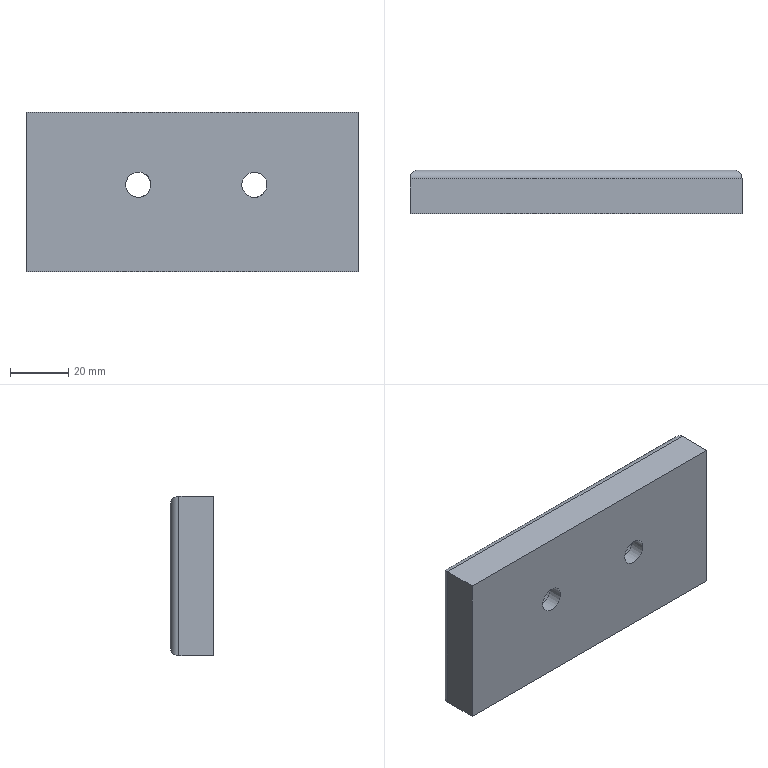Part | STEP file | 1_id1606_x_t | 1 solid | 16 faces | box 114.3 x 15 x 55 mm | volume 89525 mm3 | plane 8 | cylinder 8 | commonest cylinder face diameters 6 x4 8.7 x2 15 x2
STEP:
#1=CARTESIAN_POINT('',(0.,0.,0.));
#2=DIRECTION('',(0.,0.,1.));
#3=DIRECTION('',(1.,0.,0.));
#4=AXIS2_PLACEMENT_3D('',#1,#2,#3);
#5=CARTESIAN_POINT('',(661.35,282.376,-11.278));
#6=VERTEX_POINT('',#5);
#7=CARTESIAN_POINT('',(553.05,282.376,-11.278));
#8=VERTEX_POINT('',#7);
#9=CARTESIAN_POINT('',(661.35,282.376,-11.278));
#10=DIRECTION('',(-1.,0.,0.));
#11=VECTOR('',#10,1.);
#12=LINE('',#9,#11);
#13=CARTESIAN_POINT('',(606.2,282.376,-8.278));
#14=DIRECTION('',(0.,1.,0.));
#15=DIRECTION('',(0.,0.,-1.));
#16=AXIS2_PLACEMENT_3D('',#13,#14,#15);
#17=PLANE('',#16);
#18=CARTESIAN_POINT('',(3.,-55.15));
#19=DIRECTION('',(0.,1.));
#20=VECTOR('',#19,1.);
#21=LINE('',#18,#20);
#22=(GEOMETRIC_REPRESENTATION_CONTEXT(2)PARAMETRIC_REPRESENTATION_CONTEXT()REPRESENTATION_CONTEXT('',''));
#23=DEFINITIONAL_REPRESENTATION('',(#21),#22);
#24=PCURVE('',#17,#23);
#25=CARTESIAN_POINT('',(606.2,279.376,-11.278));
#26=DIRECTION('',(1.,0.,0.));
#27=DIRECTION('',(0.,0.,-1.));
#28=AXIS2_PLACEMENT_3D('',#25,#26,#27);
#29=CYLINDRICAL_SURFACE('',#28,3.);
#30=CARTESIAN_POINT('',(1.571,55.15));
#31=DIRECTION('',(0.,-1.));
#32=VECTOR('',#31,1.);
#33=LINE('',#30,#32);
#34=(GEOMETRIC_REPRESENTATION_CONTEXT(2)PARAMETRIC_REPRESENTATION_CONTEXT()REPRESENTATION_CONTEXT('',''));
#35=DEFINITIONAL_REPRESENTATION('',(#33),#34);
#36=PCURVE('',#29,#35);
#37=SURFACE_CURVE('',#12,(#24,#36),.PCURVE_S1.);
#38=EDGE_CURVE('',#6,#8,#37,.T.);
#39=ORIENTED_EDGE('',*,*,#38,.F.);
#40=CARTESIAN_POINT('',(661.35,282.376,-60.278));
#41=VERTEX_POINT('',#40);
#42=CARTESIAN_POINT('',(661.35,282.376,-60.278));
#43=DIRECTION('',(0.,0.,1.));
#44=VECTOR('',#43,1.);
#45=LINE('',#42,#44);
#46=CARTESIAN_POINT('',(52.,-55.15));
#47=DIRECTION('',(-1.,0.));
#48=VECTOR('',#47,1.);
#49=LINE('',#46,#48);
#50=(GEOMETRIC_REPRESENTATION_CONTEXT(2)PARAMETRIC_REPRESENTATION_CONTEXT()REPRESENTATION_CONTEXT('',''));
#51=DEFINITIONAL_REPRESENTATION('',(#49),#50);
#52=PCURVE('',#17,#51);
#53=CARTESIAN_POINT('',(661.35,279.376,-8.278));
#54=DIRECTION('',(0.,0.,-1.));
#55=DIRECTION('',(-1.,0.,0.));
#56=AXIS2_PLACEMENT_3D('',#53,#54,#55);
#57=CYLINDRICAL_SURFACE('',#56,3.);
#58=CARTESIAN_POINT('',(1.571,52.));
#59=DIRECTION('',(0.,-1.));
#60=VECTOR('',#59,1.);
#61=LINE('',#58,#60);
#62=(GEOMETRIC_REPRESENTATION_CONTEXT(2)PARAMETRIC_REPRESENTATION_CONTEXT()REPRESENTATION_CONTEXT('',''));
#63=DEFINITIONAL_REPRESENTATION('',(#61),#62);
#64=PCURVE('',#57,#63);
#65=SURFACE_CURVE('',#45,(#52,#64),.PCURVE_S1.);
#66=EDGE_CURVE('',#41,#6,#65,.T.);
#67=ORIENTED_EDGE('',*,*,#66,.F.);
#68=CARTESIAN_POINT('',(553.05,282.376,-60.278));
#69=VERTEX_POINT('',#68);
#70=CARTESIAN_POINT('',(553.05,282.376,-60.278));
#71=DIRECTION('',(1.,0.,0.));
#72=VECTOR('',#71,1.);
#73=LINE('',#70,#72);
#74=CARTESIAN_POINT('',(52.,53.15));
#75=DIRECTION('',(0.,-1.));
#76=VECTOR('',#75,1.);
#77=LINE('',#74,#76);
#78=(GEOMETRIC_REPRESENTATION_CONTEXT(2)PARAMETRIC_REPRESENTATION_CONTEXT()REPRESENTATION_CONTEXT('',''));
#79=DEFINITIONAL_REPRESENTATION('',(#77),#78);
#80=PCURVE('',#17,#79);
#81=CARTESIAN_POINT('',(606.2,279.376,-60.278));
#82=DIRECTION('',(-1.,0.,0.));
#83=DIRECTION('',(0.,0.,1.));
#84=AXIS2_PLACEMENT_3D('',#81,#82,#83);
#85=CYLINDRICAL_SURFACE('',#84,3.);
#86=CARTESIAN_POINT('',(1.571,53.15));
#87=DIRECTION('',(0.,-1.));
#88=VECTOR('',#87,1.);
#89=LINE('',#86,#88);
#90=(GEOMETRIC_REPRESENTATION_CONTEXT(2)PARAMETRIC_REPRESENTATION_CONTEXT()REPRESENTATION_CONTEXT('',''));
#91=DEFINITIONAL_REPRESENTATION('',(#89),#90);
#92=PCURVE('',#85,#91);
#93=SURFACE_CURVE('',#73,(#80,#92),.PCURVE_S1.);
#94=EDGE_CURVE('',#69,#41,#93,.T.);
#95=ORIENTED_EDGE('',*,*,#94,.F.);
#96=CARTESIAN_POINT('',(553.05,282.376,-11.278));
#97=DIRECTION('',(0.,0.,-1.));
#98=VECTOR('',#97,1.);
#99=LINE('',#96,#98);
#100=CARTESIAN_POINT('',(3.,53.15));
#101=DIRECTION('',(1.,0.));
#102=VECTOR('',#101,1.);
#103=LINE('',#100,#102);
#104=(GEOMETRIC_REPRESENTATION_CONTEXT(2)PARAMETRIC_REPRESENTATION_CONTEXT()REPRESENTATION_CONTEXT('',''));
#105=DEFINITIONAL_REPRESENTATION('',(#103),#104);
#106=PCURVE('',#17,#105);
#107=CARTESIAN_POINT('',(553.05,279.376,-8.278));
#108=DIRECTION('',(0.,0.,-1.));
#109=DIRECTION('',(-1.,0.,0.));
#110=AXIS2_PLACEMENT_3D('',#107,#108,#109);
#111=CYLINDRICAL_SURFACE('',#110,3.);
#112=CARTESIAN_POINT('',(1.571,3.));
#113=DIRECTION('',(0.,1.));
#114=VECTOR('',#113,1.);
#115=LINE('',#112,#114);
#116=(GEOMETRIC_REPRESENTATION_CONTEXT(2)PARAMETRIC_REPRESENTATION_CONTEXT()REPRESENTATION_CONTEXT('',''));
#117=DEFINITIONAL_REPRESENTATION('',(#115),#116);
#118=PCURVE('',#111,#117);
#119=SURFACE_CURVE('',#99,(#106,#118),.PCURVE_S1.);
#120=EDGE_CURVE('',#8,#69,#119,.T.);
#121=ORIENTED_EDGE('',*,*,#120,.F.);
#122=EDGE_LOOP('',(#39,#67,#95,#121));
#123=FACE_BOUND('',#122,.T.);
#124=CARTESIAN_POINT('',(628.7,282.376,-25.778));
#125=VERTEX_POINT('',#124);
#126=CARTESIAN_POINT('',(628.7,282.376,-33.278));
#127=DIRECTION('',(0.,-1.,0.));
#128=DIRECTION('',(0.,0.,1.));
#129=AXIS2_PLACEMENT_3D('',#126,#127,#128);
#130=CIRCLE('',#129,7.5);
#131=CARTESIAN_POINT('',(17.5,-22.5));
#132=CARTESIAN_POINT('',(17.5,-9.51));
#133=CARTESIAN_POINT('',(28.75,-16.005));
#134=CARTESIAN_POINT('',(40.,-22.5));
#135=CARTESIAN_POINT('',(28.75,-28.995));
#136=CARTESIAN_POINT('',(17.5,-35.49));
#137=CARTESIAN_POINT('',(17.5,-22.5));
#138=(BOUNDED_CURVE()B_SPLINE_CURVE(2,(#131,#132,#133,#134,#135,#136,#137),.UNSPECIFIED.,.T.,.F.)B_SPLINE_CURVE_WITH_KNOTS((1,2,2,2,2,1),(-2.094,0.,2.094,4.189,6.283,8.378),.UNSPECIFIED.)CURVE()GEOMETRIC_REPRESENTATION_ITEM()RATIONAL_B_SPLINE_CURVE((1.,0.5,1.,0.5,1.,0.5,1.))REPRESENTATION_ITEM(''));
#139=(GEOMETRIC_REPRESENTATION_CONTEXT(2)PARAMETRIC_REPRESENTATION_CONTEXT()REPRESENTATION_CONTEXT('',''));
#140=DEFINITIONAL_REPRESENTATION('',(#138),#139);
#141=PCURVE('',#17,#140);
#142=CARTESIAN_POINT('',(628.7,272.376,-33.278));
#143=DIRECTION('',(0.,-1.,0.));
#144=DIRECTION('',(1.,0.,0.));
#145=AXIS2_PLACEMENT_3D('',#142,#143,#144);
#146=CYLINDRICAL_SURFACE('',#145,7.5);
#147=CARTESIAN_POINT('',(1.571,-10.));
#148=DIRECTION('',(1.,0.));
#149=VECTOR('',#148,1.);
#150=LINE('',#147,#149);
#151=(GEOMETRIC_REPRESENTATION_CONTEXT(2)PARAMETRIC_REPRESENTATION_CONTEXT()REPRESENTATION_CONTEXT('',''));
#152=DEFINITIONAL_REPRESENTATION('',(#150),#151);
#153=PCURVE('',#146,#152);
#154=SURFACE_CURVE('',#130,(#141,#153),.PCURVE_S1.);
#155=EDGE_CURVE('',#125,#125,#154,.T.);
#156=ORIENTED_EDGE('',*,*,#155,.T.);
#157=EDGE_LOOP('',(#156));
#158=FACE_BOUND('',#157,.T.);
#159=CARTESIAN_POINT('',(581.2,282.376,-33.278));
#160=VERTEX_POINT('',#159);
#161=CARTESIAN_POINT('',(588.7,282.376,-33.278));
#162=DIRECTION('',(0.,-1.,0.));
#163=DIRECTION('',(-1.,0.,0.));
#164=AXIS2_PLACEMENT_3D('',#161,#162,#163);
#165=CIRCLE('',#164,7.5);
#166=CARTESIAN_POINT('',(25.,25.));
#167=CARTESIAN_POINT('',(37.99,25.));
#168=CARTESIAN_POINT('',(31.495,13.75));
#169=CARTESIAN_POINT('',(25.,2.5));
#170=CARTESIAN_POINT('',(18.505,13.75));
#171=CARTESIAN_POINT('',(12.01,25.));
#172=CARTESIAN_POINT('',(25.,25.));
#173=(BOUNDED_CURVE()B_SPLINE_CURVE(2,(#166,#167,#168,#169,#170,#171,#172),.UNSPECIFIED.,.T.,.F.)B_SPLINE_CURVE_WITH_KNOTS((1,2,2,2,2,1),(-2.094,0.,2.094,4.189,6.283,8.378),.UNSPECIFIED.)CURVE()GEOMETRIC_REPRESENTATION_ITEM()RATIONAL_B_SPLINE_CURVE((1.,0.5,1.,0.5,1.,0.5,1.))REPRESENTATION_ITEM(''));
#174=(GEOMETRIC_REPRESENTATION_CONTEXT(2)PARAMETRIC_REPRESENTATION_CONTEXT()REPRESENTATION_CONTEXT('',''));
#175=DEFINITIONAL_REPRESENTATION('',(#173),#174);
#176=PCURVE('',#17,#175);
#177=CARTESIAN_POINT('',(588.7,272.376,-33.278));
#178=DIRECTION('',(0.,-1.,0.));
#179=DIRECTION('',(1.,0.,0.));
#180=AXIS2_PLACEMENT_3D('',#177,#178,#179);
#181=CYLINDRICAL_SURFACE('',#180,7.5);
#182=CARTESIAN_POINT('',(3.142,-10.));
#183=DIRECTION('',(1.,0.));
#184=VECTOR('',#183,1.);
#185=LINE('',#182,#184);
#186=(GEOMETRIC_REPRESENTATION_CONTEXT(2)PARAMETRIC_REPRESENTATION_CONTEXT()REPRESENTATION_CONTEXT('',''));
#187=DEFINITIONAL_REPRESENTATION('',(#185),#186);
#188=PCURVE('',#181,#187);
#189=SURFACE_CURVE('',#165,(#176,#188),.PCURVE_S1.);
#190=EDGE_CURVE('',#160,#160,#189,.T.);
#191=ORIENTED_EDGE('',*,*,#190,.T.);
#192=EDGE_LOOP('',(#191));
#193=FACE_BOUND('',#192,.T.);
#194=ADVANCED_FACE('',(#123,#158,#193),#17,.T.);
#195=CARTESIAN_POINT('',(550.05,279.376,-63.278));
#196=VERTEX_POINT('',#195);
#197=CARTESIAN_POINT('',(550.05,279.376,-8.278));
#198=VERTEX_POINT('',#197);
#199=CARTESIAN_POINT('',(550.05,279.376,-63.278));
#200=DIRECTION('',(0.,0.,1.));
#201=VECTOR('',#200,1.);
#202=LINE('',#199,#201);
#203=CARTESIAN_POINT('',(0.,55.));
#204=DIRECTION('',(0.,-1.));
#205=VECTOR('',#204,1.);
#206=LINE('',#203,#205);
#207=(GEOMETRIC_REPRESENTATION_CONTEXT(2)PARAMETRIC_REPRESENTATION_CONTEXT()REPRESENTATION_CONTEXT('',''));
#208=DEFINITIONAL_REPRESENTATION('',(#206),#207);
#209=PCURVE('',#111,#208);
#210=CARTESIAN_POINT('',(550.05,274.876,-8.278));
#211=DIRECTION('',(-1.,0.,0.));
#212=DIRECTION('',(0.,0.,1.));
#213=AXIS2_PLACEMENT_3D('',#210,#211,#212);
#214=PLANE('',#213);
#215=CARTESIAN_POINT('',(-55.,4.5));
#216=DIRECTION('',(1.,0.));
#217=VECTOR('',#216,1.);
#218=LINE('',#215,#217);
#219=(GEOMETRIC_REPRESENTATION_CONTEXT(2)PARAMETRIC_REPRESENTATION_CONTEXT()REPRESENTATION_CONTEXT('',''));
#220=DEFINITIONAL_REPRESENTATION('',(#218),#219);
#221=PCURVE('',#214,#220);
#222=SURFACE_CURVE('',#202,(#209,#221),.PCURVE_S1.);
#223=EDGE_CURVE('',#196,#198,#222,.T.);
#224=ORIENTED_EDGE('',*,*,#223,.T.);
#225=CARTESIAN_POINT('',(553.05,279.376,-11.278));
#226=DIRECTION('',(-0.7071,0.,-0.7071));
#227=DIRECTION('',(0.7071,0.,-0.7071));
#228=AXIS2_PLACEMENT_3D('',#225,#226,#227);
#229=ELLIPSE('',#228,4.243,3.);
#230=CARTESIAN_POINT('',(0.,0.));
#231=CARTESIAN_POINT('',(0.0238,-0.00000647));
#232=CARTESIAN_POINT('',(0.0714,0.005103));
#233=CARTESIAN_POINT('',(0.1428,0.02801));
#234=CARTESIAN_POINT('',(0.2142,0.06607));
#235=CARTESIAN_POINT('',(0.2856,0.1191));
#236=CARTESIAN_POINT('',(0.357,0.1868));
#237=CARTESIAN_POINT('',(0.4284,0.2688));
#238=CARTESIAN_POINT('',(0.4998,0.3647));
#239=CARTESIAN_POINT('',(0.5712,0.4741));
#240=CARTESIAN_POINT('',(0.6426,0.5963));
#241=CARTESIAN_POINT('',(0.714,0.7308));
#242=CARTESIAN_POINT('',(0.7854,0.8769));
#243=CARTESIAN_POINT('',(0.8568,1.034));
#244=CARTESIAN_POINT('',(0.9282,1.201));
#245=CARTESIAN_POINT('',(0.9996,1.377));
#246=CARTESIAN_POINT('',(1.071,1.561));
#247=CARTESIAN_POINT('',(1.142,1.753));
#248=CARTESIAN_POINT('',(1.214,1.951));
#249=CARTESIAN_POINT('',(1.285,2.154));
#250=CARTESIAN_POINT('',(1.357,2.362));
#251=CARTESIAN_POINT('',(1.428,2.573));
#252=CARTESIAN_POINT('',(1.499,2.786));
#253=CARTESIAN_POINT('',(1.547,2.929));
#254=CARTESIAN_POINT('',(1.571,3.));
#255=B_SPLINE_CURVE_WITH_KNOTS('',3,(#230,#231,#232,#233,#234,#235,#236,#237,#238,#239,#240,#241,#242,#243,#244,#245,#246,#247,#248,#249,#250,#251,#252,#253,#254),.UNSPECIFIED.,.F.,.F.,(4,1,1,1,1,1,1,1,1,1,1,1,1,1,1,1,1,1,1,1,1,1,4),(3.142,3.213,3.284,3.356,3.427,3.499,3.57,3.641,3.713,3.784,3.856,3.927,3.998,4.07,4.141,4.213,4.284,4.355,4.427,4.498,4.57,4.641,4.712),.QUASI_UNIFORM_KNOTS.);
#256=(GEOMETRIC_REPRESENTATION_CONTEXT(2)PARAMETRIC_REPRESENTATION_CONTEXT()REPRESENTATION_CONTEXT('',''));
#257=DEFINITIONAL_REPRESENTATION('',(#255),#256);
#258=PCURVE('',#111,#257);
#259=CARTESIAN_POINT('',(3.142,-56.15));
#260=CARTESIAN_POINT('',(3.118,-56.15));
#261=CARTESIAN_POINT('',(3.07,-56.145));
#262=CARTESIAN_POINT('',(2.999,-56.122));
#263=CARTESIAN_POINT('',(2.927,-56.084));
#264=CARTESIAN_POINT('',(2.856,-56.031));
#265=CARTESIAN_POINT('',(2.785,-55.963));
#266=CARTESIAN_POINT('',(2.713,-55.881));
#267=CARTESIAN_POINT('',(2.642,-55.785));
#268=CARTESIAN_POINT('',(2.57,-55.676));
#269=CARTESIAN_POINT('',(2.499,-55.554));
#270=CARTESIAN_POINT('',(2.428,-55.419));
#271=CARTESIAN_POINT('',(2.356,-55.273));
#272=CARTESIAN_POINT('',(2.285,-55.116));
#273=CARTESIAN_POINT('',(2.213,-54.949));
#274=CARTESIAN_POINT('',(2.142,-54.773));
#275=CARTESIAN_POINT('',(2.071,-54.589));
#276=CARTESIAN_POINT('',(1.999,-54.397));
#277=CARTESIAN_POINT('',(1.928,-54.199));
#278=CARTESIAN_POINT('',(1.856,-53.996));
#279=CARTESIAN_POINT('',(1.785,-53.788));
#280=CARTESIAN_POINT('',(1.714,-53.577));
#281=CARTESIAN_POINT('',(1.642,-53.364));
#282=CARTESIAN_POINT('',(1.595,-53.221));
#283=CARTESIAN_POINT('',(1.571,-53.15));
#284=B_SPLINE_CURVE_WITH_KNOTS('',3,(#259,#260,#261,#262,#263,#264,#265,#266,#267,#268,#269,#270,#271,#272,#273,#274,#275,#276,#277,#278,#279,#280,#281,#282,#283),.UNSPECIFIED.,.F.,.F.,(4,1,1,1,1,1,1,1,1,1,1,1,1,1,1,1,1,1,1,1,1,1,4),(3.142,3.213,3.284,3.356,3.427,3.499,3.57,3.641,3.713,3.784,3.856,3.927,3.998,4.07,4.141,4.213,4.284,4.355,4.427,4.498,4.57,4.641,4.712),.QUASI_UNIFORM_KNOTS.);
#285=(GEOMETRIC_REPRESENTATION_CONTEXT(2)PARAMETRIC_REPRESENTATION_CONTEXT()REPRESENTATION_CONTEXT('',''));
#286=DEFINITIONAL_REPRESENTATION('',(#284),#285);
#287=PCURVE('',#29,#286);
#288=SURFACE_CURVE('',#229,(#258,#287),.PCURVE_S1.);
#289=EDGE_CURVE('',#198,#8,#288,.T.);
#290=ORIENTED_EDGE('',*,*,#289,.T.);
#291=ORIENTED_EDGE('',*,*,#120,.T.);
#292=CARTESIAN_POINT('',(553.05,279.376,-60.278));
#293=DIRECTION('',(0.7071,0.,-0.7071));
#294=DIRECTION('',(-0.7071,0.,-0.7071));
#295=AXIS2_PLACEMENT_3D('',#292,#293,#294);
#296=ELLIPSE('',#295,4.243,3.);
#297=CARTESIAN_POINT('',(0.,55.));
#298=CARTESIAN_POINT('',(0.0238,55.));
#299=CARTESIAN_POINT('',(0.0714,54.995));
#300=CARTESIAN_POINT('',(0.1428,54.972));
#301=CARTESIAN_POINT('',(0.2142,54.934));
#302=CARTESIAN_POINT('',(0.2856,54.881));
#303=CARTESIAN_POINT('',(0.357,54.813));
#304=CARTESIAN_POINT('',(0.4284,54.731));
#305=CARTESIAN_POINT('',(0.4998,54.635));
#306=CARTESIAN_POINT('',(0.5712,54.526));
#307=CARTESIAN_POINT('',(0.6426,54.404));
#308=CARTESIAN_POINT('',(0.714,54.269));
#309=CARTESIAN_POINT('',(0.7854,54.123));
#310=CARTESIAN_POINT('',(0.8568,53.966));
#311=CARTESIAN_POINT('',(0.9282,53.799));
#312=CARTESIAN_POINT('',(0.9996,53.623));
#313=CARTESIAN_POINT('',(1.071,53.439));
#314=CARTESIAN_POINT('',(1.142,53.247));
#315=CARTESIAN_POINT('',(1.214,53.049));
#316=CARTESIAN_POINT('',(1.285,52.846));
#317=CARTESIAN_POINT('',(1.357,52.638));
#318=CARTESIAN_POINT('',(1.428,52.427));
#319=CARTESIAN_POINT('',(1.499,52.214));
#320=CARTESIAN_POINT('',(1.547,52.071));
#321=CARTESIAN_POINT('',(1.571,52.));
#322=B_SPLINE_CURVE_WITH_KNOTS('',3,(#297,#298,#299,#300,#301,#302,#303,#304,#305,#306,#307,#308,#309,#310,#311,#312,#313,#314,#315,#316,#317,#318,#319,#320,#321),.UNSPECIFIED.,.F.,.F.,(4,1,1,1,1,1,1,1,1,1,1,1,1,1,1,1,1,1,1,1,1,1,4),(0.,0.0714,0.1428,0.2142,0.2856,0.357,0.4284,0.4998,0.5712,0.6426,0.714,0.7854,0.8568,0.9282,0.9996,1.071,1.142,1.214,1.285,1.357,1.428,1.499,1.571),.QUASI_UNIFORM_KNOTS.);
#323=(GEOMETRIC_REPRESENTATION_CONTEXT(2)PARAMETRIC_REPRESENTATION_CONTEXT()REPRESENTATION_CONTEXT('',''));
#324=DEFINITIONAL_REPRESENTATION('',(#322),#323);
#325=PCURVE('',#111,#324);
#326=CARTESIAN_POINT('',(3.142,56.15));
#327=CARTESIAN_POINT('',(3.118,56.15));
#328=CARTESIAN_POINT('',(3.07,56.145));
#329=CARTESIAN_POINT('',(2.999,56.122));
#330=CARTESIAN_POINT('',(2.927,56.084));
#331=CARTESIAN_POINT('',(2.856,56.031));
#332=CARTESIAN_POINT('',(2.785,55.963));
#333=CARTESIAN_POINT('',(2.713,55.881));
#334=CARTESIAN_POINT('',(2.642,55.785));
#335=CARTESIAN_POINT('',(2.57,55.676));
#336=CARTESIAN_POINT('',(2.499,55.554));
#337=CARTESIAN_POINT('',(2.428,55.419));
#338=CARTESIAN_POINT('',(2.356,55.273));
#339=CARTESIAN_POINT('',(2.285,55.116));
#340=CARTESIAN_POINT('',(2.213,54.949));
#341=CARTESIAN_POINT('',(2.142,54.773));
#342=CARTESIAN_POINT('',(2.071,54.589));
#343=CARTESIAN_POINT('',(1.999,54.397));
#344=CARTESIAN_POINT('',(1.928,54.199));
#345=CARTESIAN_POINT('',(1.856,53.996));
#346=CARTESIAN_POINT('',(1.785,53.788));
#347=CARTESIAN_POINT('',(1.714,53.577));
#348=CARTESIAN_POINT('',(1.642,53.364));
#349=CARTESIAN_POINT('',(1.595,53.221));
#350=CARTESIAN_POINT('',(1.571,53.15));
#351=B_SPLINE_CURVE_WITH_KNOTS('',3,(#326,#327,#328,#329,#330,#331,#332,#333,#334,#335,#336,#337,#338,#339,#340,#341,#342,#343,#344,#345,#346,#347,#348,#349,#350),.UNSPECIFIED.,.F.,.F.,(4,1,1,1,1,1,1,1,1,1,1,1,1,1,1,1,1,1,1,1,1,1,4),(0.,0.0714,0.1428,0.2142,0.2856,0.357,0.4284,0.4998,0.5712,0.6426,0.714,0.7854,0.8568,0.9282,0.9996,1.071,1.142,1.214,1.285,1.357,1.428,1.499,1.571),.QUASI_UNIFORM_KNOTS.);
#352=(GEOMETRIC_REPRESENTATION_CONTEXT(2)PARAMETRIC_REPRESENTATION_CONTEXT()REPRESENTATION_CONTEXT('',''));
#353=DEFINITIONAL_REPRESENTATION('',(#351),#352);
#354=PCURVE('',#85,#353);
#355=SURFACE_CURVE('',#296,(#325,#354),.PCURVE_S1.);
#356=EDGE_CURVE('',#196,#69,#355,.T.);
#357=ORIENTED_EDGE('',*,*,#356,.F.);
#358=EDGE_LOOP('',(#224,#290,#291,#357));
#359=FACE_BOUND('',#358,.T.);
#360=ADVANCED_FACE('',(#359),#111,.T.);
#361=CARTESIAN_POINT('',(664.35,279.376,-63.278));
#362=VERTEX_POINT('',#361);
#363=CARTESIAN_POINT('',(664.35,279.376,-63.278));
#364=DIRECTION('',(-1.,0.,0.));
#365=VECTOR('',#364,1.);
#366=LINE('',#363,#365);
#367=CARTESIAN_POINT('',(3.142,-58.15));
#368=DIRECTION('',(0.,1.));
#369=VECTOR('',#368,1.);
#370=LINE('',#367,#369);
#371=(GEOMETRIC_REPRESENTATION_CONTEXT(2)PARAMETRIC_REPRESENTATION_CONTEXT()REPRESENTATION_CONTEXT('',''));
#372=DEFINITIONAL_REPRESENTATION('',(#370),#371);
#373=PCURVE('',#85,#372);
#374=CARTESIAN_POINT('',(606.2,274.876,-63.278));
#375=DIRECTION('',(0.,0.,-1.));
#376=DIRECTION('',(-1.,0.,0.));
#377=AXIS2_PLACEMENT_3D('',#374,#375,#376);
#378=PLANE('',#377);
#379=CARTESIAN_POINT('',(-58.15,4.5));
#380=DIRECTION('',(1.,0.));
#381=VECTOR('',#380,1.);
#382=LINE('',#379,#381);
#383=(GEOMETRIC_REPRESENTATION_CONTEXT(2)PARAMETRIC_REPRESENTATION_CONTEXT()REPRESENTATION_CONTEXT('',''));
#384=DEFINITIONAL_REPRESENTATION('',(#382),#383);
#385=PCURVE('',#378,#384);
#386=SURFACE_CURVE('',#366,(#373,#385),.PCURVE_S1.);
#387=EDGE_CURVE('',#362,#196,#386,.T.);
#388=ORIENTED_EDGE('',*,*,#387,.T.);
#389=ORIENTED_EDGE('',*,*,#356,.T.);
#390=ORIENTED_EDGE('',*,*,#94,.T.);
#391=CARTESIAN_POINT('',(661.35,279.376,-60.278));
#392=DIRECTION('',(0.7071,0.,0.7071));
#393=DIRECTION('',(0.7071,0.,-0.7071));
#394=AXIS2_PLACEMENT_3D('',#391,#392,#393);
#395=ELLIPSE('',#394,4.243,3.);
#396=CARTESIAN_POINT('',(3.142,-58.15));
#397=CARTESIAN_POINT('',(3.118,-58.15));
#398=CARTESIAN_POINT('',(3.07,-58.145));
#399=CARTESIAN_POINT('',(2.999,-58.122));
#400=CARTESIAN_POINT('',(2.927,-58.084));
#401=CARTESIAN_POINT('',(2.856,-58.031));
#402=CARTESIAN_POINT('',(2.785,-57.963));
#403=CARTESIAN_POINT('',(2.713,-57.881));
#404=CARTESIAN_POINT('',(2.642,-57.785));
#405=CARTESIAN_POINT('',(2.57,-57.676));
#406=CARTESIAN_POINT('',(2.499,-57.554));
#407=CARTESIAN_POINT('',(2.428,-57.419));
#408=CARTESIAN_POINT('',(2.356,-57.273));
#409=CARTESIAN_POINT('',(2.285,-57.116));
#410=CARTESIAN_POINT('',(2.213,-56.949));
#411=CARTESIAN_POINT('',(2.142,-56.773));
#412=CARTESIAN_POINT('',(2.071,-56.589));
#413=CARTESIAN_POINT('',(1.999,-56.397));
#414=CARTESIAN_POINT('',(1.928,-56.199));
#415=CARTESIAN_POINT('',(1.856,-55.996));
#416=CARTESIAN_POINT('',(1.785,-55.788));
#417=CARTESIAN_POINT('',(1.714,-55.577));
#418=CARTESIAN_POINT('',(1.642,-55.364));
#419=CARTESIAN_POINT('',(1.595,-55.221));
#420=CARTESIAN_POINT('',(1.571,-55.15));
#421=B_SPLINE_CURVE_WITH_KNOTS('',3,(#396,#397,#398,#399,#400,#401,#402,#403,#404,#405,#406,#407,#408,#409,#410,#411,#412,#413,#414,#415,#416,#417,#418,#419,#420),.UNSPECIFIED.,.F.,.F.,(4,1,1,1,1,1,1,1,1,1,1,1,1,1,1,1,1,1,1,1,1,1,4),(0.,0.0714,0.1428,0.2142,0.2856,0.357,0.4284,0.4998,0.5712,0.6426,0.714,0.7854,0.8568,0.9282,0.9996,1.071,1.142,1.214,1.285,1.357,1.428,1.499,1.571),.QUASI_UNIFORM_KNOTS.);
#422=(GEOMETRIC_REPRESENTATION_CONTEXT(2)PARAMETRIC_REPRESENTATION_CONTEXT()REPRESENTATION_CONTEXT('',''));
#423=DEFINITIONAL_REPRESENTATION('',(#421),#422);
#424=PCURVE('',#85,#423);
#425=CARTESIAN_POINT('',(3.142,55.));
#426=CARTESIAN_POINT('',(3.118,55.));
#427=CARTESIAN_POINT('',(3.07,54.995));
#428=CARTESIAN_POINT('',(2.999,54.972));
#429=CARTESIAN_POINT('',(2.927,54.934));
#430=CARTESIAN_POINT('',(2.856,54.881));
#431=CARTESIAN_POINT('',(2.785,54.813));
#432=CARTESIAN_POINT('',(2.713,54.731));
#433=CARTESIAN_POINT('',(2.642,54.635));
#434=CARTESIAN_POINT('',(2.57,54.526));
#435=CARTESIAN_POINT('',(2.499,54.404));
#436=CARTESIAN_POINT('',(2.428,54.269));
#437=CARTESIAN_POINT('',(2.356,54.123));
#438=CARTESIAN_POINT('',(2.285,53.966));
#439=CARTESIAN_POINT('',(2.213,53.799));
#440=CARTESIAN_POINT('',(2.142,53.623));
#441=CARTESIAN_POINT('',(2.071,53.439));
#442=CARTESIAN_POINT('',(1.999,53.247));
#443=CARTESIAN_POINT('',(1.928,53.049));
#444=CARTESIAN_POINT('',(1.856,52.846));
#445=CARTESIAN_POINT('',(1.785,52.638));
#446=CARTESIAN_POINT('',(1.714,52.427));
#447=CARTESIAN_POINT('',(1.642,52.214));
#448=CARTESIAN_POINT('',(1.595,52.071));
#449=CARTESIAN_POINT('',(1.571,52.));
#450=B_SPLINE_CURVE_WITH_KNOTS('',3,(#425,#426,#427,#428,#429,#430,#431,#432,#433,#434,#435,#436,#437,#438,#439,#440,#441,#442,#443,#444,#445,#446,#447,#448,#449),.UNSPECIFIED.,.F.,.F.,(4,1,1,1,1,1,1,1,1,1,1,1,1,1,1,1,1,1,1,1,1,1,4),(0.,0.0714,0.1428,0.2142,0.2856,0.357,0.4284,0.4998,0.5712,0.6426,0.714,0.7854,0.8568,0.9282,0.9996,1.071,1.142,1.214,1.285,1.357,1.428,1.499,1.571),.QUASI_UNIFORM_KNOTS.);
#451=(GEOMETRIC_REPRESENTATION_CONTEXT(2)PARAMETRIC_REPRESENTATION_CONTEXT()REPRESENTATION_CONTEXT('',''));
#452=DEFINITIONAL_REPRESENTATION('',(#450),#451);
#453=PCURVE('',#57,#452);
#454=SURFACE_CURVE('',#395,(#424,#453),.PCURVE_S1.);
#455=EDGE_CURVE('',#362,#41,#454,.T.);
#456=ORIENTED_EDGE('',*,*,#455,.F.);
#457=EDGE_LOOP('',(#388,#389,#390,#456));
#458=FACE_BOUND('',#457,.T.);
#459=ADVANCED_FACE('',(#458),#85,.T.);
#460=ORIENTED_EDGE('',*,*,#66,.T.);
#461=CARTESIAN_POINT('',(664.35,279.376,-8.278));
#462=VERTEX_POINT('',#461);
#463=CARTESIAN_POINT('',(661.35,279.376,-11.278));
#464=DIRECTION('',(-0.7071,0.,0.7071));
#465=DIRECTION('',(0.7071,0.,0.7071));
#466=AXIS2_PLACEMENT_3D('',#463,#464,#465);
#467=ELLIPSE('',#466,4.243,3.);
#468=CARTESIAN_POINT('',(3.142,0.));
#469=CARTESIAN_POINT('',(3.118,-0.00000647));
#470=CARTESIAN_POINT('',(3.07,0.005103));
#471=CARTESIAN_POINT('',(2.999,0.02801));
#472=CARTESIAN_POINT('',(2.927,0.06607));
#473=CARTESIAN_POINT('',(2.856,0.1191));
#474=CARTESIAN_POINT('',(2.785,0.1868));
#475=CARTESIAN_POINT('',(2.713,0.2688));
#476=CARTESIAN_POINT('',(2.642,0.3647));
#477=CARTESIAN_POINT('',(2.57,0.4741));
#478=CARTESIAN_POINT('',(2.499,0.5963));
#479=CARTESIAN_POINT('',(2.428,0.7308));
#480=CARTESIAN_POINT('',(2.356,0.8769));
#481=CARTESIAN_POINT('',(2.285,1.034));
#482=CARTESIAN_POINT('',(2.213,1.201));
#483=CARTESIAN_POINT('',(2.142,1.377));
#484=CARTESIAN_POINT('',(2.071,1.561));
#485=CARTESIAN_POINT('',(1.999,1.753));
#486=CARTESIAN_POINT('',(1.928,1.951));
#487=CARTESIAN_POINT('',(1.856,2.154));
#488=CARTESIAN_POINT('',(1.785,2.362));
#489=CARTESIAN_POINT('',(1.714,2.573));
#490=CARTESIAN_POINT('',(1.642,2.786));
#491=CARTESIAN_POINT('',(1.595,2.929));
#492=CARTESIAN_POINT('',(1.571,3.));
#493=B_SPLINE_CURVE_WITH_KNOTS('',3,(#468,#469,#470,#471,#472,#473,#474,#475,#476,#477,#478,#479,#480,#481,#482,#483,#484,#485,#486,#487,#488,#489,#490,#491,#492),.UNSPECIFIED.,.F.,.F.,(4,1,1,1,1,1,1,1,1,1,1,1,1,1,1,1,1,1,1,1,1,1,4),(0.,0.0714,0.1428,0.2142,0.2856,0.357,0.4284,0.4998,0.5712,0.6426,0.714,0.7854,0.8568,0.9282,0.9996,1.071,1.142,1.214,1.285,1.357,1.428,1.499,1.571),.QUASI_UNIFORM_KNOTS.);
#494=(GEOMETRIC_REPRESENTATION_CONTEXT(2)PARAMETRIC_REPRESENTATION_CONTEXT()REPRESENTATION_CONTEXT('',''));
#495=DEFINITIONAL_REPRESENTATION('',(#493),#494);
#496=PCURVE('',#57,#495);
#497=CARTESIAN_POINT('',(3.142,58.15));
#498=CARTESIAN_POINT('',(3.118,58.15));
#499=CARTESIAN_POINT('',(3.07,58.145));
#500=CARTESIAN_POINT('',(2.999,58.122));
#501=CARTESIAN_POINT('',(2.927,58.084));
#502=CARTESIAN_POINT('',(2.856,58.031));
#503=CARTESIAN_POINT('',(2.785,57.963));
#504=CARTESIAN_POINT('',(2.713,57.881));
#505=CARTESIAN_POINT('',(2.642,57.785));
#506=CARTESIAN_POINT('',(2.57,57.676));
#507=CARTESIAN_POINT('',(2.499,57.554));
#508=CARTESIAN_POINT('',(2.428,57.419));
#509=CARTESIAN_POINT('',(2.356,57.273));
#510=CARTESIAN_POINT('',(2.285,57.116));
#511=CARTESIAN_POINT('',(2.213,56.949));
#512=CARTESIAN_POINT('',(2.142,56.773));
#513=CARTESIAN_POINT('',(2.071,56.589));
#514=CARTESIAN_POINT('',(1.999,56.397));
#515=CARTESIAN_POINT('',(1.928,56.199));
#516=CARTESIAN_POINT('',(1.856,55.996));
#517=CARTESIAN_POINT('',(1.785,55.788));
#518=CARTESIAN_POINT('',(1.714,55.577));
#519=CARTESIAN_POINT('',(1.642,55.364));
#520=CARTESIAN_POINT('',(1.595,55.221));
#521=CARTESIAN_POINT('',(1.571,55.15));
#522=B_SPLINE_CURVE_WITH_KNOTS('',3,(#497,#498,#499,#500,#501,#502,#503,#504,#505,#506,#507,#508,#509,#510,#511,#512,#513,#514,#515,#516,#517,#518,#519,#520,#521),.UNSPECIFIED.,.F.,.F.,(4,1,1,1,1,1,1,1,1,1,1,1,1,1,1,1,1,1,1,1,1,1,4),(0.,0.0714,0.1428,0.2142,0.2856,0.357,0.4284,0.4998,0.5712,0.6426,0.714,0.7854,0.8568,0.9282,0.9996,1.071,1.142,1.214,1.285,1.357,1.428,1.499,1.571),.QUASI_UNIFORM_KNOTS.);
#523=(GEOMETRIC_REPRESENTATION_CONTEXT(2)PARAMETRIC_REPRESENTATION_CONTEXT()REPRESENTATION_CONTEXT('',''));
#524=DEFINITIONAL_REPRESENTATION('',(#522),#523);
#525=PCURVE('',#29,#524);
#526=SURFACE_CURVE('',#467,(#496,#525),.PCURVE_S1.);
#527=EDGE_CURVE('',#462,#6,#526,.T.);
#528=ORIENTED_EDGE('',*,*,#527,.F.);
#529=CARTESIAN_POINT('',(664.35,279.376,-8.278));
#530=DIRECTION('',(0.,0.,-1.));
#531=VECTOR('',#530,1.);
#532=LINE('',#529,#531);
#533=CARTESIAN_POINT('',(3.142,0.));
#534=DIRECTION('',(0.,1.));
#535=VECTOR('',#534,1.);
#536=LINE('',#533,#535);
#537=(GEOMETRIC_REPRESENTATION_CONTEXT(2)PARAMETRIC_REPRESENTATION_CONTEXT()REPRESENTATION_CONTEXT('',''));
#538=DEFINITIONAL_REPRESENTATION('',(#536),#537);
#539=PCURVE('',#57,#538);
#540=CARTESIAN_POINT('',(664.35,274.876,-8.278));
#541=DIRECTION('',(1.,0.,0.));
#542=DIRECTION('',(0.,0.,-1.));
#543=AXIS2_PLACEMENT_3D('',#540,#541,#542);
#544=PLANE('',#543);
#545=CARTESIAN_POINT('',(0.,4.5));
#546=DIRECTION('',(1.,0.));
#547=VECTOR('',#546,1.);
#548=LINE('',#545,#547);
#549=(GEOMETRIC_REPRESENTATION_CONTEXT(2)PARAMETRIC_REPRESENTATION_CONTEXT()REPRESENTATION_CONTEXT('',''));
#550=DEFINITIONAL_REPRESENTATION('',(#548),#549);
#551=PCURVE('',#544,#550);
#552=SURFACE_CURVE('',#532,(#539,#551),.PCURVE_S1.);
#553=EDGE_CURVE('',#462,#362,#552,.T.);
#554=ORIENTED_EDGE('',*,*,#553,.T.);
#555=ORIENTED_EDGE('',*,*,#455,.T.);
#556=EDGE_LOOP('',(#460,#528,#554,#555));
#557=FACE_BOUND('',#556,.T.);
#558=ADVANCED_FACE('',(#557),#57,.T.);
#559=ORIENTED_EDGE('',*,*,#553,.F.);
#560=CARTESIAN_POINT('',(664.35,267.376,-8.278));
#561=VERTEX_POINT('',#560);
#562=CARTESIAN_POINT('',(664.35,267.376,-8.278));
#563=DIRECTION('',(0.,1.,0.));
#564=VECTOR('',#563,1.);
#565=LINE('',#562,#564);
#566=CARTESIAN_POINT('',(0.,-7.5));
#567=DIRECTION('',(0.,1.));
#568=VECTOR('',#567,1.);
#569=LINE('',#566,#568);
#570=(GEOMETRIC_REPRESENTATION_CONTEXT(2)PARAMETRIC_REPRESENTATION_CONTEXT()REPRESENTATION_CONTEXT('',''));
#571=DEFINITIONAL_REPRESENTATION('',(#569),#570);
#572=PCURVE('',#544,#571);
#573=CARTESIAN_POINT('',(606.2,274.876,-8.278));
#574=DIRECTION('',(0.,0.,1.));
#575=DIRECTION('',(1.,0.,0.));
#576=AXIS2_PLACEMENT_3D('',#573,#574,#575);
#577=PLANE('',#576);
#578=CARTESIAN_POINT('',(58.15,-7.5));
#579=DIRECTION('',(0.,1.));
#580=VECTOR('',#579,1.);
#581=LINE('',#578,#580);
#582=(GEOMETRIC_REPRESENTATION_CONTEXT(2)PARAMETRIC_REPRESENTATION_CONTEXT()REPRESENTATION_CONTEXT('',''));
#583=DEFINITIONAL_REPRESENTATION('',(#581),#582);
#584=PCURVE('',#577,#583);
#585=SURFACE_CURVE('',#565,(#572,#584),.PCURVE_S1.);
#586=EDGE_CURVE('',#561,#462,#585,.T.);
#587=ORIENTED_EDGE('',*,*,#586,.F.);
#588=CARTESIAN_POINT('',(664.35,267.376,-63.278));
#589=VERTEX_POINT('',#588);
#590=CARTESIAN_POINT('',(664.35,267.376,-63.278));
#591=DIRECTION('',(0.,0.,1.));
#592=VECTOR('',#591,1.);
#593=LINE('',#590,#592);
#594=CARTESIAN_POINT('',(55.,-7.5));
#595=DIRECTION('',(-1.,0.));
#596=VECTOR('',#595,1.);
#597=LINE('',#594,#596);
#598=(GEOMETRIC_REPRESENTATION_CONTEXT(2)PARAMETRIC_REPRESENTATION_CONTEXT()REPRESENTATION_CONTEXT('',''));
#599=DEFINITIONAL_REPRESENTATION('',(#597),#598);
#600=PCURVE('',#544,#599);
#601=CARTESIAN_POINT('',(606.2,267.376,-8.278));
#602=DIRECTION('',(0.,-1.,0.));
#603=DIRECTION('',(0.,0.,1.));
#604=AXIS2_PLACEMENT_3D('',#601,#602,#603);
#605=PLANE('',#604);
#606=CARTESIAN_POINT('',(-55.,-58.15));
#607=DIRECTION('',(1.,0.));
#608=VECTOR('',#607,1.);
#609=LINE('',#606,#608);
#610=(GEOMETRIC_REPRESENTATION_CONTEXT(2)PARAMETRIC_REPRESENTATION_CONTEXT()REPRESENTATION_CONTEXT('',''));
#611=DEFINITIONAL_REPRESENTATION('',(#609),#610);
#612=PCURVE('',#605,#611);
#613=SURFACE_CURVE('',#593,(#600,#612),.PCURVE_S1.);
#614=EDGE_CURVE('',#589,#561,#613,.T.);
#615=ORIENTED_EDGE('',*,*,#614,.F.);
#616=CARTESIAN_POINT('',(664.35,279.376,-63.278));
#617=DIRECTION('',(0.,-1.,0.));
#618=VECTOR('',#617,1.);
#619=LINE('',#616,#618);
#620=CARTESIAN_POINT('',(55.,4.5));
#621=DIRECTION('',(0.,-1.));
#622=VECTOR('',#621,1.);
#623=LINE('',#620,#622);
#624=(GEOMETRIC_REPRESENTATION_CONTEXT(2)PARAMETRIC_REPRESENTATION_CONTEXT()REPRESENTATION_CONTEXT('',''));
#625=DEFINITIONAL_REPRESENTATION('',(#623),#624);
#626=PCURVE('',#544,#625);
#627=CARTESIAN_POINT('',(-58.15,4.5));
#628=DIRECTION('',(0.,-1.));
#629=VECTOR('',#628,1.);
#630=LINE('',#627,#629);
#631=(GEOMETRIC_REPRESENTATION_CONTEXT(2)PARAMETRIC_REPRESENTATION_CONTEXT()REPRESENTATION_CONTEXT('',''));
#632=DEFINITIONAL_REPRESENTATION('',(#630),#631);
#633=PCURVE('',#378,#632);
#634=SURFACE_CURVE('',#619,(#626,#633),.PCURVE_S1.);
#635=EDGE_CURVE('',#362,#589,#634,.T.);
#636=ORIENTED_EDGE('',*,*,#635,.F.);
#637=EDGE_LOOP('',(#559,#587,#615,#636));
#638=FACE_BOUND('',#637,.T.);
#639=ADVANCED_FACE('',(#638),#544,.T.);
#640=ORIENTED_EDGE('',*,*,#387,.F.);
#641=ORIENTED_EDGE('',*,*,#635,.T.);
#642=CARTESIAN_POINT('',(550.05,267.376,-63.278));
#643=VERTEX_POINT('',#642);
#644=CARTESIAN_POINT('',(664.35,267.376,-63.278));
#645=DIRECTION('',(-1.,0.,0.));
#646=VECTOR('',#645,1.);
#647=LINE('',#644,#646);
#648=CARTESIAN_POINT('',(-58.15,-7.5));
#649=DIRECTION('',(1.,0.));
#650=VECTOR('',#649,1.);
#651=LINE('',#648,#650);
#652=(GEOMETRIC_REPRESENTATION_CONTEXT(2)PARAMETRIC_REPRESENTATION_CONTEXT()REPRESENTATION_CONTEXT('',''));
#653=DEFINITIONAL_REPRESENTATION('',(#651),#652);
#654=PCURVE('',#378,#653);
#655=CARTESIAN_POINT('',(-55.,-58.15));
#656=DIRECTION('',(0.,1.));
#657=VECTOR('',#656,1.);
#658=LINE('',#655,#657);
#659=(GEOMETRIC_REPRESENTATION_CONTEXT(2)PARAMETRIC_REPRESENTATION_CONTEXT()REPRESENTATION_CONTEXT('',''));
#660=DEFINITIONAL_REPRESENTATION('',(#658),#659);
#661=PCURVE('',#605,#660);
#662=SURFACE_CURVE('',#647,(#654,#661),.PCURVE_S1.);
#663=EDGE_CURVE('',#589,#643,#662,.T.);
#664=ORIENTED_EDGE('',*,*,#663,.T.);
#665=CARTESIAN_POINT('',(550.05,267.376,-63.278));
#666=DIRECTION('',(0.,1.,0.));
#667=VECTOR('',#666,1.);
#668=LINE('',#665,#667);
#669=CARTESIAN_POINT('',(56.15,-7.5));
#670=DIRECTION('',(0.,1.));
#671=VECTOR('',#670,1.);
#672=LINE('',#669,#671);
#673=(GEOMETRIC_REPRESENTATION_CONTEXT(2)PARAMETRIC_REPRESENTATION_CONTEXT()REPRESENTATION_CONTEXT('',''));
#674=DEFINITIONAL_REPRESENTATION('',(#672),#673);
#675=PCURVE('',#378,#674);
#676=CARTESIAN_POINT('',(-55.,-7.5));
#677=DIRECTION('',(0.,1.));
#678=VECTOR('',#677,1.);
#679=LINE('',#676,#678);
#680=(GEOMETRIC_REPRESENTATION_CONTEXT(2)PARAMETRIC_REPRESENTATION_CONTEXT()REPRESENTATION_CONTEXT('',''));
#681=DEFINITIONAL_REPRESENTATION('',(#679),#680);
#682=PCURVE('',#214,#681);
#683=SURFACE_CURVE('',#668,(#675,#682),.PCURVE_S1.);
#684=EDGE_CURVE('',#643,#196,#683,.T.);
#685=ORIENTED_EDGE('',*,*,#684,.T.);
#686=EDGE_LOOP('',(#640,#641,#664,#685));
#687=FACE_BOUND('',#686,.T.);
#688=ADVANCED_FACE('',(#687),#378,.T.);
#689=ORIENTED_EDGE('',*,*,#223,.F.);
#690=ORIENTED_EDGE('',*,*,#684,.F.);
#691=CARTESIAN_POINT('',(550.05,267.376,-8.278));
#692=VERTEX_POINT('',#691);
#693=CARTESIAN_POINT('',(550.05,267.376,-63.278));
#694=DIRECTION('',(0.,0.,1.));
#695=VECTOR('',#694,1.);
#696=LINE('',#693,#695);
#697=CARTESIAN_POINT('',(-55.,-7.5));
#698=DIRECTION('',(1.,0.));
#699=VECTOR('',#698,1.);
#700=LINE('',#697,#699);
#701=(GEOMETRIC_REPRESENTATION_CONTEXT(2)PARAMETRIC_REPRESENTATION_CONTEXT()REPRESENTATION_CONTEXT('',''));
#702=DEFINITIONAL_REPRESENTATION('',(#700),#701);
#703=PCURVE('',#214,#702);
#704=CARTESIAN_POINT('',(-55.,56.15));
#705=DIRECTION('',(1.,0.));
#706=VECTOR('',#705,1.);
#707=LINE('',#704,#706);
#708=(GEOMETRIC_REPRESENTATION_CONTEXT(2)PARAMETRIC_REPRESENTATION_CONTEXT()REPRESENTATION_CONTEXT('',''));
#709=DEFINITIONAL_REPRESENTATION('',(#707),#708);
#710=PCURVE('',#605,#709);
#711=SURFACE_CURVE('',#696,(#703,#710),.PCURVE_S1.);
#712=EDGE_CURVE('',#643,#692,#711,.T.);
#713=ORIENTED_EDGE('',*,*,#712,.T.);
#714=CARTESIAN_POINT('',(550.05,279.376,-8.278));
#715=DIRECTION('',(0.,-1.,0.));
#716=VECTOR('',#715,1.);
#717=LINE('',#714,#716);
#718=CARTESIAN_POINT('',(0.,4.5));
#719=DIRECTION('',(0.,-1.));
#720=VECTOR('',#719,1.);
#721=LINE('',#718,#720);
#722=(GEOMETRIC_REPRESENTATION_CONTEXT(2)PARAMETRIC_REPRESENTATION_CONTEXT()REPRESENTATION_CONTEXT('',''));
#723=DEFINITIONAL_REPRESENTATION('',(#721),#722);
#724=PCURVE('',#214,#723);
#725=CARTESIAN_POINT('',(-56.15,4.5));
#726=DIRECTION('',(0.,-1.));
#727=VECTOR('',#726,1.);
#728=LINE('',#725,#727);
#729=(GEOMETRIC_REPRESENTATION_CONTEXT(2)PARAMETRIC_REPRESENTATION_CONTEXT()REPRESENTATION_CONTEXT('',''));
#730=DEFINITIONAL_REPRESENTATION('',(#728),#729);
#731=PCURVE('',#577,#730);
#732=SURFACE_CURVE('',#717,(#724,#731),.PCURVE_S1.);
#733=EDGE_CURVE('',#198,#692,#732,.T.);
#734=ORIENTED_EDGE('',*,*,#733,.F.);
#735=EDGE_LOOP('',(#689,#690,#713,#734));
#736=FACE_BOUND('',#735,.T.);
#737=ADVANCED_FACE('',(#736),#214,.T.);
#738=CARTESIAN_POINT('',(550.05,279.376,-8.278));
#739=DIRECTION('',(1.,0.,0.));
#740=VECTOR('',#739,1.);
#741=LINE('',#738,#740);
#742=CARTESIAN_POINT('',(-56.15,4.5));
#743=DIRECTION('',(1.,0.));
#744=VECTOR('',#743,1.);
#745=LINE('',#742,#744);
#746=(GEOMETRIC_REPRESENTATION_CONTEXT(2)PARAMETRIC_REPRESENTATION_CONTEXT()REPRESENTATION_CONTEXT('',''));
#747=DEFINITIONAL_REPRESENTATION('',(#745),#746);
#748=PCURVE('',#577,#747);
#749=CARTESIAN_POINT('',(3.142,-56.15));
#750=DIRECTION('',(0.,1.));
#751=VECTOR('',#750,1.);
#752=LINE('',#749,#751);
#753=(GEOMETRIC_REPRESENTATION_CONTEXT(2)PARAMETRIC_REPRESENTATION_CONTEXT()REPRESENTATION_CONTEXT('',''));
#754=DEFINITIONAL_REPRESENTATION('',(#752),#753);
#755=PCURVE('',#29,#754);
#756=SURFACE_CURVE('',#741,(#748,#755),.PCURVE_S1.);
#757=EDGE_CURVE('',#198,#462,#756,.T.);
#758=ORIENTED_EDGE('',*,*,#757,.F.);
#759=ORIENTED_EDGE('',*,*,#733,.T.);
#760=CARTESIAN_POINT('',(550.05,267.376,-8.278));
#761=DIRECTION('',(1.,0.,0.));
#762=VECTOR('',#761,1.);
#763=LINE('',#760,#762);
#764=CARTESIAN_POINT('',(-56.15,-7.5));
#765=DIRECTION('',(1.,0.));
#766=VECTOR('',#765,1.);
#767=LINE('',#764,#766);
#768=(GEOMETRIC_REPRESENTATION_CONTEXT(2)PARAMETRIC_REPRESENTATION_CONTEXT()REPRESENTATION_CONTEXT('',''));
#769=DEFINITIONAL_REPRESENTATION('',(#767),#768);
#770=PCURVE('',#577,#769);
#771=CARTESIAN_POINT('',(0.,56.15));
#772=DIRECTION('',(0.,-1.));
#773=VECTOR('',#772,1.);
#774=LINE('',#771,#773);
#775=(GEOMETRIC_REPRESENTATION_CONTEXT(2)PARAMETRIC_REPRESENTATION_CONTEXT()REPRESENTATION_CONTEXT('',''));
#776=DEFINITIONAL_REPRESENTATION('',(#774),#775);
#777=PCURVE('',#605,#776);
#778=SURFACE_CURVE('',#763,(#770,#777),.PCURVE_S1.);
#779=EDGE_CURVE('',#692,#561,#778,.T.);
#780=ORIENTED_EDGE('',*,*,#779,.T.);
#781=ORIENTED_EDGE('',*,*,#586,.T.);
#782=EDGE_LOOP('',(#758,#759,#780,#781));
#783=FACE_BOUND('',#782,.T.);
#784=ADVANCED_FACE('',(#783),#577,.T.);
#785=ORIENTED_EDGE('',*,*,#663,.F.);
#786=ORIENTED_EDGE('',*,*,#614,.T.);
#787=ORIENTED_EDGE('',*,*,#779,.F.);
#788=ORIENTED_EDGE('',*,*,#712,.F.);
#789=EDGE_LOOP('',(#785,#786,#787,#788));
#790=FACE_BOUND('',#789,.T.);
#791=CARTESIAN_POINT('',(628.7,267.376,-37.628));
#792=VERTEX_POINT('',#791);
#793=CARTESIAN_POINT('',(628.7,267.376,-33.278));
#794=DIRECTION('',(0.,1.,0.));
#795=DIRECTION('',(0.,0.,-1.));
#796=AXIS2_PLACEMENT_3D('',#793,#794,#795);
#797=CIRCLE('',#796,4.35);
#798=CARTESIAN_POINT('',(-29.35,-22.5));
#799=CARTESIAN_POINT('',(-29.35,-14.966));
#800=CARTESIAN_POINT('',(-22.825,-18.733));
#801=CARTESIAN_POINT('',(-16.3,-22.5));
#802=CARTESIAN_POINT('',(-22.825,-26.267));
#803=CARTESIAN_POINT('',(-29.35,-30.034));
#804=CARTESIAN_POINT('',(-29.35,-22.5));
#805=(BOUNDED_CURVE()B_SPLINE_CURVE(2,(#798,#799,#800,#801,#802,#803,#804),.UNSPECIFIED.,.T.,.F.)B_SPLINE_CURVE_WITH_KNOTS((1,2,2,2,2,1),(-2.094,0.,2.094,4.189,6.283,8.378),.UNSPECIFIED.)CURVE()GEOMETRIC_REPRESENTATION_ITEM()RATIONAL_B_SPLINE_CURVE((1.,0.5,1.,0.5,1.,0.5,1.))REPRESENTATION_ITEM(''));
#806=(GEOMETRIC_REPRESENTATION_CONTEXT(2)PARAMETRIC_REPRESENTATION_CONTEXT()REPRESENTATION_CONTEXT('',''));
#807=DEFINITIONAL_REPRESENTATION('',(#805),#806);
#808=PCURVE('',#605,#807);
#809=CARTESIAN_POINT('',(628.7,267.226,-33.278));
#810=DIRECTION('',(0.,-1.,0.));
#811=DIRECTION('',(1.,0.,0.));
#812=AXIS2_PLACEMENT_3D('',#809,#810,#811);
#813=CYLINDRICAL_SURFACE('',#812,4.35);
#814=CARTESIAN_POINT('',(10.996,-0.15));
#815=DIRECTION('',(-1.,0.));
#816=VECTOR('',#815,1.);
#817=LINE('',#814,#816);
#818=(GEOMETRIC_REPRESENTATION_CONTEXT(2)PARAMETRIC_REPRESENTATION_CONTEXT()REPRESENTATION_CONTEXT('',''));
#819=DEFINITIONAL_REPRESENTATION('',(#817),#818);
#820=PCURVE('',#813,#819);
#821=SURFACE_CURVE('',#797,(#808,#820),.PCURVE_S1.);
#822=EDGE_CURVE('',#792,#792,#821,.T.);
#823=ORIENTED_EDGE('',*,*,#822,.T.);
#824=EDGE_LOOP('',(#823));
#825=FACE_BOUND('',#824,.T.);
#826=CARTESIAN_POINT('',(588.7,267.376,-28.928));
#827=VERTEX_POINT('',#826);
#828=CARTESIAN_POINT('',(593.05,267.376,-33.278));
#829=VERTEX_POINT('',#828);
#830=CARTESIAN_POINT('',(588.7,267.376,-33.278));
#831=DIRECTION('',(0.,1.,0.));
#832=DIRECTION('',(0.,0.,1.));
#833=AXIS2_PLACEMENT_3D('',#830,#831,#832);
#834=CIRCLE('',#833,4.35);
#835=CARTESIAN_POINT('',(-20.65,17.5));
#836=CARTESIAN_POINT('',(-20.65,9.966));
#837=CARTESIAN_POINT('',(-27.175,13.733));
#838=CARTESIAN_POINT('',(-33.7,17.5));
#839=CARTESIAN_POINT('',(-27.175,21.267));
#840=CARTESIAN_POINT('',(-20.65,25.034));
#841=CARTESIAN_POINT('',(-20.65,17.5));
#842=(BOUNDED_CURVE()B_SPLINE_CURVE(2,(#835,#836,#837,#838,#839,#840,#841),.UNSPECIFIED.,.T.,.F.)B_SPLINE_CURVE_WITH_KNOTS((1,2,2,2,2,1),(-2.094,0.,2.094,4.189,6.283,8.378),.UNSPECIFIED.)CURVE()GEOMETRIC_REPRESENTATION_ITEM()RATIONAL_B_SPLINE_CURVE((1.,0.5,1.,0.5,1.,0.5,1.))REPRESENTATION_ITEM(''));
#843=(GEOMETRIC_REPRESENTATION_CONTEXT(2)PARAMETRIC_REPRESENTATION_CONTEXT()REPRESENTATION_CONTEXT('',''));
#844=DEFINITIONAL_REPRESENTATION('',(#842),#843);
#845=PCURVE('',#605,#844);
#846=CARTESIAN_POINT('',(588.7,267.226,-33.278));
#847=DIRECTION('',(0.,-1.,0.));
#848=DIRECTION('',(1.,0.,0.));
#849=AXIS2_PLACEMENT_3D('',#846,#847,#848);
#850=CYLINDRICAL_SURFACE('',#849,4.35);
#851=CARTESIAN_POINT('',(1.571,-0.15));
#852=DIRECTION('',(-1.,0.));
#853=VECTOR('',#852,1.);
#854=LINE('',#851,#853);
#855=(GEOMETRIC_REPRESENTATION_CONTEXT(2)PARAMETRIC_REPRESENTATION_CONTEXT()REPRESENTATION_CONTEXT('',''));
#856=DEFINITIONAL_REPRESENTATION('',(#854),#855);
#857=PCURVE('',#850,#856);
#858=SURFACE_CURVE('',#834,(#845,#857),.PCURVE_S1.);
#859=EDGE_CURVE('',#827,#829,#858,.T.);
#860=ORIENTED_EDGE('',*,*,#859,.T.);
#861=CARTESIAN_POINT('',(588.7,267.376,-33.278));
#862=DIRECTION('',(0.,1.,0.));
#863=DIRECTION('',(0.,0.,1.));
#864=AXIS2_PLACEMENT_3D('',#861,#862,#863);
#865=CIRCLE('',#864,4.35);
#866=CARTESIAN_POINT('',(-20.65,17.5));
#867=CARTESIAN_POINT('',(-20.65,9.966));
#868=CARTESIAN_POINT('',(-27.175,13.733));
#869=CARTESIAN_POINT('',(-33.7,17.5));
#870=CARTESIAN_POINT('',(-27.175,21.267));
#871=CARTESIAN_POINT('',(-20.65,25.034));
#872=CARTESIAN_POINT('',(-20.65,17.5));
#873=(BOUNDED_CURVE()B_SPLINE_CURVE(2,(#866,#867,#868,#869,#870,#871,#872),.UNSPECIFIED.,.T.,.F.)B_SPLINE_CURVE_WITH_KNOTS((1,2,2,2,2,1),(-2.094,0.,2.094,4.189,6.283,8.378),.UNSPECIFIED.)CURVE()GEOMETRIC_REPRESENTATION_ITEM()RATIONAL_B_SPLINE_CURVE((1.,0.5,1.,0.5,1.,0.5,1.))REPRESENTATION_ITEM(''));
#874=(GEOMETRIC_REPRESENTATION_CONTEXT(2)PARAMETRIC_REPRESENTATION_CONTEXT()REPRESENTATION_CONTEXT('',''));
#875=DEFINITIONAL_REPRESENTATION('',(#873),#874);
#876=PCURVE('',#605,#875);
#877=CARTESIAN_POINT('',(7.854,-0.15));
#878=DIRECTION('',(-1.,0.));
#879=VECTOR('',#878,1.);
#880=LINE('',#877,#879);
#881=(GEOMETRIC_REPRESENTATION_CONTEXT(2)PARAMETRIC_REPRESENTATION_CONTEXT()REPRESENTATION_CONTEXT('',''));
#882=DEFINITIONAL_REPRESENTATION('',(#880),#881);
#883=PCURVE('',#850,#882);
#884=SURFACE_CURVE('',#865,(#876,#883),.PCURVE_S1.);
#885=EDGE_CURVE('',#829,#827,#884,.T.);
#886=ORIENTED_EDGE('',*,*,#885,.T.);
#887=EDGE_LOOP('',(#860,#886));
#888=FACE_BOUND('',#887,.T.);
#889=ADVANCED_FACE('',(#790,#825,#888),#605,.T.);
#890=ORIENTED_EDGE('',*,*,#822,.T.);
#891=CARTESIAN_POINT('',(628.7,272.376,-37.628));
#892=VERTEX_POINT('',#891);
#893=CARTESIAN_POINT('',(628.7,272.376,-37.628));
#894=CARTESIAN_POINT('',(628.7,267.376,-37.628));
#895=B_SPLINE_CURVE_WITH_KNOTS('',1,(#893,#894),.UNSPECIFIED.,.F.,.F.,(2,2),(-5.15,-0.15),.PIECEWISE_BEZIER_KNOTS.);
#896=CARTESIAN_POINT('',(4.712,0.));
#897=DIRECTION('',(0.,1.));
#898=VECTOR('',#897,1.);
#899=LINE('',#896,#898);
#900=(GEOMETRIC_REPRESENTATION_CONTEXT(2)PARAMETRIC_REPRESENTATION_CONTEXT()REPRESENTATION_CONTEXT('',''));
#901=DEFINITIONAL_REPRESENTATION('',(#899),#900);
#902=PCURVE('',#813,#901);
#903=CARTESIAN_POINT('',(10.996,0.));
#904=DIRECTION('',(0.,1.));
#905=VECTOR('',#904,1.);
#906=LINE('',#903,#905);
#907=(GEOMETRIC_REPRESENTATION_CONTEXT(2)PARAMETRIC_REPRESENTATION_CONTEXT()REPRESENTATION_CONTEXT('',''));
#908=DEFINITIONAL_REPRESENTATION('',(#906),#907);
#909=PCURVE('',#813,#908);
#910=SEAM_CURVE('',#895,(#902,#909),.PCURVE_S1.);
#911=EDGE_CURVE('',#892,#792,#910,.T.);
#912=ORIENTED_EDGE('',*,*,#911,.F.);
#913=CARTESIAN_POINT('',(624.35,272.376,-33.278));
#914=VERTEX_POINT('',#913);
#915=CARTESIAN_POINT('',(628.7,272.376,-33.278));
#916=DIRECTION('',(0.,-1.,0.));
#917=DIRECTION('',(-1.,0.,0.));
#918=AXIS2_PLACEMENT_3D('',#915,#916,#917);
#919=CIRCLE('',#918,4.35);
#920=CARTESIAN_POINT('',(3.142,-5.15));
#921=DIRECTION('',(1.,0.));
#922=VECTOR('',#921,1.);
#923=LINE('',#920,#922);
#924=(GEOMETRIC_REPRESENTATION_CONTEXT(2)PARAMETRIC_REPRESENTATION_CONTEXT()REPRESENTATION_CONTEXT('',''));
#925=DEFINITIONAL_REPRESENTATION('',(#923),#924);
#926=PCURVE('',#813,#925);
#927=CARTESIAN_POINT('',(631.7,272.376,-33.278));
#928=DIRECTION('',(0.,-1.,0.));
#929=DIRECTION('',(-1.,0.,0.));
#930=AXIS2_PLACEMENT_3D('',#927,#928,#929);
#931=PLANE('',#930);
#932=CARTESIAN_POINT('',(3.,0.));
#933=DIRECTION('',(1.,0.));
#934=AXIS2_PLACEMENT_2D('',#932,#933);
#935=CIRCLE('',#934,4.35);
#936=(GEOMETRIC_REPRESENTATION_CONTEXT(2)PARAMETRIC_REPRESENTATION_CONTEXT()REPRESENTATION_CONTEXT('',''));
#937=DEFINITIONAL_REPRESENTATION('',(#935),#936);
#938=PCURVE('',#931,#937);
#939=SURFACE_CURVE('',#919,(#926,#938),.PCURVE_S1.);
#940=EDGE_CURVE('',#892,#914,#939,.T.);
#941=ORIENTED_EDGE('',*,*,#940,.T.);
#942=CARTESIAN_POINT('',(628.7,272.376,-33.278));
#943=DIRECTION('',(0.,-1.,0.));
#944=DIRECTION('',(-1.,0.,0.));
#945=AXIS2_PLACEMENT_3D('',#942,#943,#944);
#946=CIRCLE('',#945,4.35);
#947=CARTESIAN_POINT('',(9.425,-5.15));
#948=DIRECTION('',(1.,0.));
#949=VECTOR('',#948,1.);
#950=LINE('',#947,#949);
#951=(GEOMETRIC_REPRESENTATION_CONTEXT(2)PARAMETRIC_REPRESENTATION_CONTEXT()REPRESENTATION_CONTEXT('',''));
#952=DEFINITIONAL_REPRESENTATION('',(#950),#951);
#953=PCURVE('',#813,#952);
#954=CARTESIAN_POINT('',(3.,0.));
#955=DIRECTION('',(1.,0.));
#956=AXIS2_PLACEMENT_2D('',#954,#955);
#957=CIRCLE('',#956,4.35);
#958=(GEOMETRIC_REPRESENTATION_CONTEXT(2)PARAMETRIC_REPRESENTATION_CONTEXT()REPRESENTATION_CONTEXT('',''));
#959=DEFINITIONAL_REPRESENTATION('',(#957),#958);
#960=PCURVE('',#931,#959);
#961=SURFACE_CURVE('',#946,(#953,#960),.PCURVE_S1.);
#962=EDGE_CURVE('',#914,#892,#961,.T.);
#963=ORIENTED_EDGE('',*,*,#962,.T.);
#964=ORIENTED_EDGE('',*,*,#911,.T.);
#965=EDGE_LOOP('',(#890,#912,#941,#963,#964));
#966=FACE_BOUND('',#965,.F.);
#967=ADVANCED_FACE('',(#966),#813,.F.);
#968=CARTESIAN_POINT('',(621.2,272.376,-33.278));
#969=VERTEX_POINT('',#968);
#970=CARTESIAN_POINT('',(628.7,272.376,-25.778));
#971=VERTEX_POINT('',#970);
#972=CARTESIAN_POINT('',(628.7,272.376,-33.278));
#973=DIRECTION('',(0.,1.,0.));
#974=DIRECTION('',(-1.,0.,0.));
#975=AXIS2_PLACEMENT_3D('',#972,#973,#974);
#976=CIRCLE('',#975,7.5);
#977=CARTESIAN_POINT('',(10.5,0.));
#978=CARTESIAN_POINT('',(10.5,-12.99));
#979=CARTESIAN_POINT('',(-0.75,-6.495));
#980=CARTESIAN_POINT('',(-12.,0.));
#981=CARTESIAN_POINT('',(-0.75,6.495));
#982=CARTESIAN_POINT('',(10.5,12.99));
#983=CARTESIAN_POINT('',(10.5,0.));
#984=(BOUNDED_CURVE()B_SPLINE_CURVE(2,(#977,#978,#979,#980,#981,#982,#983),.UNSPECIFIED.,.T.,.F.)B_SPLINE_CURVE_WITH_KNOTS((1,2,2,2,2,1),(-2.094,0.,2.094,4.189,6.283,8.378),.UNSPECIFIED.)CURVE()GEOMETRIC_REPRESENTATION_ITEM()RATIONAL_B_SPLINE_CURVE((1.,0.5,1.,0.5,1.,0.5,1.))REPRESENTATION_ITEM(''));
#985=(GEOMETRIC_REPRESENTATION_CONTEXT(2)PARAMETRIC_REPRESENTATION_CONTEXT()REPRESENTATION_CONTEXT('',''));
#986=DEFINITIONAL_REPRESENTATION('',(#984),#985);
#987=PCURVE('',#931,#986);
#988=CARTESIAN_POINT('',(3.142,0.));
#989=DIRECTION('',(-1.,0.));
#990=VECTOR('',#989,1.);
#991=LINE('',#988,#990);
#992=(GEOMETRIC_REPRESENTATION_CONTEXT(2)PARAMETRIC_REPRESENTATION_CONTEXT()REPRESENTATION_CONTEXT('',''));
#993=DEFINITIONAL_REPRESENTATION('',(#991),#992);
#994=PCURVE('',#146,#993);
#995=SURFACE_CURVE('',#976,(#987,#994),.PCURVE_S1.);
#996=EDGE_CURVE('',#969,#971,#995,.T.);
#997=ORIENTED_EDGE('',*,*,#996,.T.);
#998=CARTESIAN_POINT('',(628.7,272.376,-33.278));
#999=DIRECTION('',(0.,1.,0.));
#1000=DIRECTION('',(-1.,0.,0.));
#1001=AXIS2_PLACEMENT_3D('',#998,#999,#1000);
#1002=CIRCLE('',#1001,7.5);
#1003=CARTESIAN_POINT('',(10.5,0.));
#1004=CARTESIAN_POINT('',(10.5,-12.99));
#1005=CARTESIAN_POINT('',(-0.75,-6.495));
#1006=CARTESIAN_POINT('',(-12.,0.));
#1007=CARTESIAN_POINT('',(-0.75,6.495));
#1008=CARTESIAN_POINT('',(10.5,12.99));
#1009=CARTESIAN_POINT('',(10.5,0.));
#1010=(BOUNDED_CURVE()B_SPLINE_CURVE(2,(#1003,#1004,#1005,#1006,#1007,#1008,#1009),.UNSPECIFIED.,.T.,.F.)B_SPLINE_CURVE_WITH_KNOTS((1,2,2,2,2,1),(-2.094,0.,2.094,4.189,6.283,8.378),.UNSPECIFIED.)CURVE()GEOMETRIC_REPRESENTATION_ITEM()RATIONAL_B_SPLINE_CURVE((1.,0.5,1.,0.5,1.,0.5,1.))REPRESENTATION_ITEM(''));
#1011=(GEOMETRIC_REPRESENTATION_CONTEXT(2)PARAMETRIC_REPRESENTATION_CONTEXT()REPRESENTATION_CONTEXT('',''));
#1012=DEFINITIONAL_REPRESENTATION('',(#1010),#1011);
#1013=PCURVE('',#931,#1012);
#1014=CARTESIAN_POINT('',(9.425,0.));
#1015=DIRECTION('',(-1.,0.));
#1016=VECTOR('',#1015,1.);
#1017=LINE('',#1014,#1016);
#1018=(GEOMETRIC_REPRESENTATION_CONTEXT(2)PARAMETRIC_REPRESENTATION_CONTEXT()REPRESENTATION_CONTEXT('',''));
#1019=DEFINITIONAL_REPRESENTATION('',(#1017),#1018);
#1020=PCURVE('',#146,#1019);
#1021=SURFACE_CURVE('',#1002,(#1013,#1020),.PCURVE_S1.);
#1022=EDGE_CURVE('',#971,#969,#1021,.T.);
#1023=ORIENTED_EDGE('',*,*,#1022,.T.);
#1024=EDGE_LOOP('',(#997,#1023));
#1025=FACE_BOUND('',#1024,.T.);
#1026=ORIENTED_EDGE('',*,*,#962,.T.);
#1027=ORIENTED_EDGE('',*,*,#940,.T.);
#1028=EDGE_LOOP('',(#1026,#1027));
#1029=FACE_BOUND('',#1028,.T.);
#1030=ADVANCED_FACE('',(#1025,#1029),#931,.F.);
#1031=ORIENTED_EDGE('',*,*,#996,.T.);
#1032=CARTESIAN_POINT('',(628.7,282.376,-25.778));
#1033=CARTESIAN_POINT('',(628.7,272.376,-25.778));
#1034=B_SPLINE_CURVE_WITH_KNOTS('',1,(#1032,#1033),.UNSPECIFIED.,.F.,.F.,(2,2),(-10.,0.),.PIECEWISE_BEZIER_KNOTS.);
#1035=CARTESIAN_POINT('',(1.571,0.));
#1036=DIRECTION('',(0.,1.));
#1037=VECTOR('',#1036,1.);
#1038=LINE('',#1035,#1037);
#1039=(GEOMETRIC_REPRESENTATION_CONTEXT(2)PARAMETRIC_REPRESENTATION_CONTEXT()REPRESENTATION_CONTEXT('',''));
#1040=DEFINITIONAL_REPRESENTATION('',(#1038),#1039);
#1041=PCURVE('',#146,#1040);
#1042=CARTESIAN_POINT('',(7.854,0.));
#1043=DIRECTION('',(0.,1.));
#1044=VECTOR('',#1043,1.);
#1045=LINE('',#1042,#1044);
#1046=(GEOMETRIC_REPRESENTATION_CONTEXT(2)PARAMETRIC_REPRESENTATION_CONTEXT()REPRESENTATION_CONTEXT('',''));
#1047=DEFINITIONAL_REPRESENTATION('',(#1045),#1046);
#1048=PCURVE('',#146,#1047);
#1049=SEAM_CURVE('',#1034,(#1041,#1048),.PCURVE_S1.);
#1050=EDGE_CURVE('',#125,#971,#1049,.T.);
#1051=ORIENTED_EDGE('',*,*,#1050,.F.);
#1052=ORIENTED_EDGE('',*,*,#155,.T.);
#1053=ORIENTED_EDGE('',*,*,#1050,.T.);
#1054=ORIENTED_EDGE('',*,*,#1022,.T.);
#1055=EDGE_LOOP('',(#1031,#1051,#1052,#1053,#1054));
#1056=FACE_BOUND('',#1055,.F.);
#1057=ADVANCED_FACE('',(#1056),#146,.F.);
#1058=ORIENTED_EDGE('',*,*,#859,.T.);
#1059=CARTESIAN_POINT('',(593.05,272.376,-33.278));
#1060=VERTEX_POINT('',#1059);
#1061=CARTESIAN_POINT('',(593.05,272.376,-33.278));
#1062=CARTESIAN_POINT('',(593.05,267.376,-33.278));
#1063=B_SPLINE_CURVE_WITH_KNOTS('',1,(#1061,#1062),.UNSPECIFIED.,.F.,.F.,(2,2),(-5.15,-0.15),.PIECEWISE_BEZIER_KNOTS.);
#1064=CARTESIAN_POINT('',(0.,0.));
#1065=DIRECTION('',(0.,1.));
#1066=VECTOR('',#1065,1.);
#1067=LINE('',#1064,#1066);
#1068=(GEOMETRIC_REPRESENTATION_CONTEXT(2)PARAMETRIC_REPRESENTATION_CONTEXT()REPRESENTATION_CONTEXT('',''));
#1069=DEFINITIONAL_REPRESENTATION('',(#1067),#1068);
#1070=PCURVE('',#850,#1069);
#1071=CARTESIAN_POINT('',(6.283,0.));
#1072=DIRECTION('',(0.,1.));
#1073=VECTOR('',#1072,1.);
#1074=LINE('',#1071,#1073);
#1075=(GEOMETRIC_REPRESENTATION_CONTEXT(2)PARAMETRIC_REPRESENTATION_CONTEXT()REPRESENTATION_CONTEXT('',''));
#1076=DEFINITIONAL_REPRESENTATION('',(#1074),#1075);
#1077=PCURVE('',#850,#1076);
#1078=SEAM_CURVE('',#1063,(#1070,#1077),.PCURVE_S1.);
#1079=EDGE_CURVE('',#1060,#829,#1078,.T.);
#1080=ORIENTED_EDGE('',*,*,#1079,.F.);
#1081=CARTESIAN_POINT('',(588.7,272.376,-33.278));
#1082=DIRECTION('',(0.,-1.,0.));
#1083=DIRECTION('',(1.,0.,0.));
#1084=AXIS2_PLACEMENT_3D('',#1081,#1082,#1083);
#1085=CIRCLE('',#1084,4.35);
#1086=CARTESIAN_POINT('',(0.,-5.15));
#1087=DIRECTION('',(1.,0.));
#1088=VECTOR('',#1087,1.);
#1089=LINE('',#1086,#1088);
#1090=(GEOMETRIC_REPRESENTATION_CONTEXT(2)PARAMETRIC_REPRESENTATION_CONTEXT()REPRESENTATION_CONTEXT('',''));
#1091=DEFINITIONAL_REPRESENTATION('',(#1089),#1090);
#1092=PCURVE('',#850,#1091);
#1093=CARTESIAN_POINT('',(591.7,272.376,-33.278));
#1094=DIRECTION('',(0.,-1.,0.));
#1095=DIRECTION('',(-1.,0.,0.));
#1096=AXIS2_PLACEMENT_3D('',#1093,#1094,#1095);
#1097=PLANE('',#1096);
#1098=CARTESIAN_POINT('',(3.,0.));
#1099=DIRECTION('',(-1.,0.));
#1100=AXIS2_PLACEMENT_2D('',#1098,#1099);
#1101=CIRCLE('',#1100,4.35);
#1102=(GEOMETRIC_REPRESENTATION_CONTEXT(2)PARAMETRIC_REPRESENTATION_CONTEXT()REPRESENTATION_CONTEXT('',''));
#1103=DEFINITIONAL_REPRESENTATION('',(#1101),#1102);
#1104=PCURVE('',#1097,#1103);
#1105=SURFACE_CURVE('',#1085,(#1092,#1104),.PCURVE_S1.);
#1106=EDGE_CURVE('',#1060,#1060,#1105,.T.);
#1107=ORIENTED_EDGE('',*,*,#1106,.T.);
#1108=ORIENTED_EDGE('',*,*,#1079,.T.);
#1109=ORIENTED_EDGE('',*,*,#885,.T.);
#1110=EDGE_LOOP('',(#1058,#1080,#1107,#1108,#1109));
#1111=FACE_BOUND('',#1110,.F.);
#1112=ADVANCED_FACE('',(#1111),#850,.F.);
#1113=CARTESIAN_POINT('',(581.2,272.376,-33.278));
#1114=VERTEX_POINT('',#1113);
#1115=CARTESIAN_POINT('',(588.7,272.376,-33.278));
#1116=DIRECTION('',(0.,1.,0.));
#1117=DIRECTION('',(-1.,0.,0.));
#1118=AXIS2_PLACEMENT_3D('',#1115,#1116,#1117);
#1119=CIRCLE('',#1118,7.5);
#1120=CARTESIAN_POINT('',(10.5,0.));
#1121=CARTESIAN_POINT('',(10.5,-12.99));
#1122=CARTESIAN_POINT('',(-0.75,-6.495));
#1123=CARTESIAN_POINT('',(-12.,0.));
#1124=CARTESIAN_POINT('',(-0.75,6.495));
#1125=CARTESIAN_POINT('',(10.5,12.99));
#1126=CARTESIAN_POINT('',(10.5,0.));
#1127=(BOUNDED_CURVE()B_SPLINE_CURVE(2,(#1120,#1121,#1122,#1123,#1124,#1125,#1126),.UNSPECIFIED.,.T.,.F.)B_SPLINE_CURVE_WITH_KNOTS((1,2,2,2,2,1),(-2.094,0.,2.094,4.189,6.283,8.378),.UNSPECIFIED.)CURVE()GEOMETRIC_REPRESENTATION_ITEM()RATIONAL_B_SPLINE_CURVE((1.,0.5,1.,0.5,1.,0.5,1.))REPRESENTATION_ITEM(''));
#1128=(GEOMETRIC_REPRESENTATION_CONTEXT(2)PARAMETRIC_REPRESENTATION_CONTEXT()REPRESENTATION_CONTEXT('',''));
#1129=DEFINITIONAL_REPRESENTATION('',(#1127),#1128);
#1130=PCURVE('',#1097,#1129);
#1131=CARTESIAN_POINT('',(9.425,0.));
#1132=DIRECTION('',(-1.,0.));
#1133=VECTOR('',#1132,1.);
#1134=LINE('',#1131,#1133);
#1135=(GEOMETRIC_REPRESENTATION_CONTEXT(2)PARAMETRIC_REPRESENTATION_CONTEXT()REPRESENTATION_CONTEXT('',''));
#1136=DEFINITIONAL_REPRESENTATION('',(#1134),#1135);
#1137=PCURVE('',#181,#1136);
#1138=SURFACE_CURVE('',#1119,(#1130,#1137),.PCURVE_S1.);
#1139=EDGE_CURVE('',#1114,#1114,#1138,.T.);
#1140=ORIENTED_EDGE('',*,*,#1139,.T.);
#1141=EDGE_LOOP('',(#1140));
#1142=FACE_BOUND('',#1141,.T.);
#1143=ORIENTED_EDGE('',*,*,#1106,.T.);
#1144=EDGE_LOOP('',(#1143));
#1145=FACE_BOUND('',#1144,.T.);
#1146=ADVANCED_FACE('',(#1142,#1145),#1097,.F.);
#1147=ORIENTED_EDGE('',*,*,#1139,.T.);
#1148=CARTESIAN_POINT('',(581.2,282.376,-33.278));
#1149=CARTESIAN_POINT('',(581.2,272.376,-33.278));
#1150=B_SPLINE_CURVE_WITH_KNOTS('',1,(#1148,#1149),.UNSPECIFIED.,.F.,.F.,(2,2),(-10.,0.),.PIECEWISE_BEZIER_KNOTS.);
#1151=CARTESIAN_POINT('',(3.142,0.));
#1152=DIRECTION('',(0.,1.));
#1153=VECTOR('',#1152,1.);
#1154=LINE('',#1151,#1153);
#1155=(GEOMETRIC_REPRESENTATION_CONTEXT(2)PARAMETRIC_REPRESENTATION_CONTEXT()REPRESENTATION_CONTEXT('',''));
#1156=DEFINITIONAL_REPRESENTATION('',(#1154),#1155);
#1157=PCURVE('',#181,#1156);
#1158=CARTESIAN_POINT('',(9.425,0.));
#1159=DIRECTION('',(0.,1.));
#1160=VECTOR('',#1159,1.);
#1161=LINE('',#1158,#1160);
#1162=(GEOMETRIC_REPRESENTATION_CONTEXT(2)PARAMETRIC_REPRESENTATION_CONTEXT()REPRESENTATION_CONTEXT('',''));
#1163=DEFINITIONAL_REPRESENTATION('',(#1161),#1162);
#1164=PCURVE('',#181,#1163);
#1165=SEAM_CURVE('',#1150,(#1157,#1164),.PCURVE_S1.);
#1166=EDGE_CURVE('',#160,#1114,#1165,.T.);
#1167=ORIENTED_EDGE('',*,*,#1166,.F.);
#1168=ORIENTED_EDGE('',*,*,#190,.T.);
#1169=ORIENTED_EDGE('',*,*,#1166,.T.);
#1170=EDGE_LOOP('',(#1147,#1167,#1168,#1169));
#1171=FACE_BOUND('',#1170,.F.);
#1172=ADVANCED_FACE('',(#1171),#181,.F.);
#1173=ORIENTED_EDGE('',*,*,#757,.T.);
#1174=ORIENTED_EDGE('',*,*,#527,.T.);
#1175=ORIENTED_EDGE('',*,*,#38,.T.);
#1176=ORIENTED_EDGE('',*,*,#289,.F.);
#1177=EDGE_LOOP('',(#1173,#1174,#1175,#1176));
#1178=FACE_BOUND('',#1177,.T.);
#1179=ADVANCED_FACE('',(#1178),#29,.T.);
#1180=CLOSED_SHELL('',(#194,#360,#459,#558,#639,#688,#737,#784,#889,#967,#1030,#1057,#1112,#1146,#1172,#1179));
#1181=MANIFOLD_SOLID_BREP('',#1180);
#1182=(LENGTH_UNIT()NAMED_UNIT(*)SI_UNIT(.MILLI.,.METRE.));
#1183=UNCERTAINTY_MEASURE_WITH_UNIT(LENGTH_MEASURE(0.000002),#1182,'','');
#1184=(NAMED_UNIT(*)PLANE_ANGLE_UNIT()SI_UNIT($,.RADIAN.));
#1185=(NAMED_UNIT(*)SI_UNIT($,.STERADIAN.)SOLID_ANGLE_UNIT());
#1186=(GEOMETRIC_REPRESENTATION_CONTEXT(3)GLOBAL_UNCERTAINTY_ASSIGNED_CONTEXT((#1183))GLOBAL_UNIT_ASSIGNED_CONTEXT((#1182,#1184,#1185))REPRESENTATION_CONTEXT('',''));
#1187=ADVANCED_BREP_SHAPE_REPRESENTATION('',(#4,#1181),#1186);